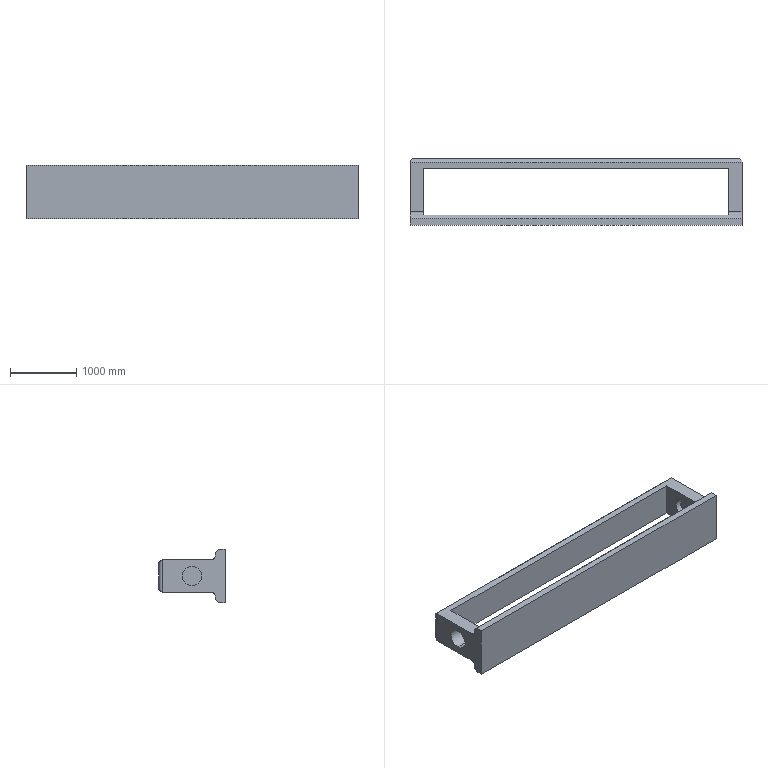Part | SolidWorks | features ICE 4, Attribute 2, Fillet 2, Chamfer 1, Extrusion 1, WeldmentFeature 1 | 1 solid | 27 faces | box 5000 x 1000 x 800 mm | volume 1070403912 mm3 | plane 17 | cylinder 10 | commonest cylinder face diameters 100 x6 290 x2 300 x2
STEP:
#1=CARTESIAN_POINT('',(4890.,500.,150.));
#2=VERTEX_POINT('',#1);
#3=CARTESIAN_POINT('',(4890.,500.,-150.));
#4=VERTEX_POINT('',#3);
#5=CARTESIAN_POINT('',(4890.,500.,0.));
#6=DIRECTION('',(1.,0.,0.));
#7=DIRECTION('',(0.,0.,-1.));
#8=AXIS2_PLACEMENT_3D('',#5,#6,#7);
#9=CIRCLE('',#8,150.);
#10=EDGE_CURVE('',#2,#4,#9,.T.);
#11=ORIENTED_EDGE('',*,*,#10,.T.);
#12=CARTESIAN_POINT('',(4800.,500.,-150.));
#13=VERTEX_POINT('',#12);
#14=CARTESIAN_POINT('',(4890.,500.,-150.));
#15=DIRECTION('',(-1.,0.,0.));
#16=VECTOR('',#15,1000.);
#17=LINE('',#14,#16);
#18=EDGE_CURVE('',#4,#13,#17,.T.);
#19=ORIENTED_EDGE('',*,*,#18,.T.);
#20=CARTESIAN_POINT('',(4800.,500.,150.));
#21=VERTEX_POINT('',#20);
#22=CARTESIAN_POINT('',(4800.,500.,0.));
#23=DIRECTION('',(1.,0.,0.));
#24=DIRECTION('',(0.,0.,-1.));
#25=AXIS2_PLACEMENT_3D('',#22,#23,#24);
#26=CIRCLE('',#25,150.);
#27=EDGE_CURVE('',#21,#13,#26,.T.);
#28=ORIENTED_EDGE('',*,*,#27,.F.);
#29=CARTESIAN_POINT('',(4890.,500.,150.));
#30=DIRECTION('',(-1.,0.,0.));
#31=VECTOR('',#30,1000.);
#32=LINE('',#29,#31);
#33=EDGE_CURVE('',#2,#21,#32,.T.);
#34=ORIENTED_EDGE('',*,*,#33,.F.);
#35=EDGE_LOOP('',(#11,#19,#28,#34));
#36=FACE_OUTER_BOUND('',#35,.T.);
#37=CARTESIAN_POINT('',(4890.,500.,0.));
#38=DIRECTION('',(-1.,0.,0.));
#39=DIRECTION('',(0.,0.,1.));
#40=AXIS2_PLACEMENT_3D('',#37,#38,#39);
#41=CYLINDRICAL_SURFACE('',#40,150.);
#42=ADVANCED_FACE('',(#36),#41,.F.);
#43=CARTESIAN_POINT('',(200.,500.,145.));
#44=VERTEX_POINT('',#43);
#45=CARTESIAN_POINT('',(200.,500.,-145.));
#46=VERTEX_POINT('',#45);
#47=CARTESIAN_POINT('',(200.,500.,0.));
#48=DIRECTION('',(1.,0.,0.));
#49=DIRECTION('',(0.,0.,1.));
#50=AXIS2_PLACEMENT_3D('',#47,#48,#49);
#51=CIRCLE('',#50,145.);
#52=EDGE_CURVE('',#44,#46,#51,.T.);
#53=ORIENTED_EDGE('',*,*,#52,.T.);
#54=CARTESIAN_POINT('',(0.,500.,-145.));
#55=VERTEX_POINT('',#54);
#56=CARTESIAN_POINT('',(610.122,500.,-145.));
#57=DIRECTION('',(-1.,0.,0.));
#58=VECTOR('',#57,1000.);
#59=LINE('',#56,#58);
#60=EDGE_CURVE('',#46,#55,#59,.T.);
#61=ORIENTED_EDGE('',*,*,#60,.T.);
#62=CARTESIAN_POINT('',(0.,500.,145.));
#63=VERTEX_POINT('',#62);
#64=CARTESIAN_POINT('',(0.,500.,0.));
#65=DIRECTION('',(1.,0.,0.));
#66=DIRECTION('',(0.,0.,-1.));
#67=AXIS2_PLACEMENT_3D('',#64,#65,#66);
#68=CIRCLE('',#67,145.);
#69=EDGE_CURVE('',#63,#55,#68,.T.);
#70=ORIENTED_EDGE('',*,*,#69,.F.);
#71=CARTESIAN_POINT('',(610.122,500.,145.));
#72=DIRECTION('',(-1.,0.,0.));
#73=VECTOR('',#72,1000.);
#74=LINE('',#71,#73);
#75=EDGE_CURVE('',#44,#63,#74,.T.);
#76=ORIENTED_EDGE('',*,*,#75,.F.);
#77=EDGE_LOOP('',(#53,#61,#70,#76));
#78=FACE_OUTER_BOUND('',#77,.T.);
#79=CARTESIAN_POINT('',(610.122,500.,0.));
#80=DIRECTION('',(-1.,0.,0.));
#81=DIRECTION('',(0.,0.,1.));
#82=AXIS2_PLACEMENT_3D('',#79,#80,#81);
#83=CYLINDRICAL_SURFACE('',#82,145.);
#84=ADVANCED_FACE('',(#78),#83,.F.);
#85=CARTESIAN_POINT('',(0.,950.,250.));
#86=VERTEX_POINT('',#85);
#87=CARTESIAN_POINT('',(0.,200.,250.));
#88=VERTEX_POINT('',#87);
#89=CARTESIAN_POINT('',(0.,1000.,250.));
#90=DIRECTION('',(0.,-1.,0.));
#91=VECTOR('',#90,1000.);
#92=LINE('',#89,#91);
#93=EDGE_CURVE('',#86,#88,#92,.T.);
#94=ORIENTED_EDGE('',*,*,#93,.T.);
#95=CARTESIAN_POINT('',(200.,200.,250.));
#96=VERTEX_POINT('',#95);
#97=CARTESIAN_POINT('',(200.,200.,250.));
#98=DIRECTION('',(1.,0.,0.));
#99=VECTOR('',#98,1000.);
#100=LINE('',#97,#99);
#101=EDGE_CURVE('',#88,#96,#100,.T.);
#102=ORIENTED_EDGE('',*,*,#101,.T.);
#103=CARTESIAN_POINT('',(200.,850.,250.));
#104=VERTEX_POINT('',#103);
#105=CARTESIAN_POINT('',(200.,850.,250.));
#106=DIRECTION('',(0.,-1.,0.));
#107=VECTOR('',#106,1000.);
#108=LINE('',#105,#107);
#109=EDGE_CURVE('',#104,#96,#108,.T.);
#110=ORIENTED_EDGE('',*,*,#109,.F.);
#111=CARTESIAN_POINT('',(4800.,850.,250.));
#112=VERTEX_POINT('',#111);
#113=CARTESIAN_POINT('',(4800.,850.,250.));
#114=DIRECTION('',(-1.,0.,0.));
#115=VECTOR('',#114,1000.);
#116=LINE('',#113,#115);
#117=EDGE_CURVE('',#112,#104,#116,.T.);
#118=ORIENTED_EDGE('',*,*,#117,.F.);
#119=CARTESIAN_POINT('',(4800.,200.,250.));
#120=VERTEX_POINT('',#119);
#121=CARTESIAN_POINT('',(4800.,850.,250.));
#122=DIRECTION('',(0.,1.,0.));
#123=VECTOR('',#122,1000.);
#124=LINE('',#121,#123);
#125=EDGE_CURVE('',#120,#112,#124,.T.);
#126=ORIENTED_EDGE('',*,*,#125,.F.);
#127=CARTESIAN_POINT('',(5000.,200.,250.));
#128=VERTEX_POINT('',#127);
#129=CARTESIAN_POINT('',(5000.,200.,250.));
#130=DIRECTION('',(1.,0.,0.));
#131=VECTOR('',#130,1000.);
#132=LINE('',#129,#131);
#133=EDGE_CURVE('',#120,#128,#132,.T.);
#134=ORIENTED_EDGE('',*,*,#133,.T.);
#135=CARTESIAN_POINT('',(5000.,950.,250.));
#136=VERTEX_POINT('',#135);
#137=CARTESIAN_POINT('',(5000.,1000.,250.));
#138=DIRECTION('',(0.,1.,0.));
#139=VECTOR('',#138,1000.);
#140=LINE('',#137,#139);
#141=EDGE_CURVE('',#128,#136,#140,.T.);
#142=ORIENTED_EDGE('',*,*,#141,.T.);
#143=CARTESIAN_POINT('',(0.,950.,250.));
#144=DIRECTION('',(-1.,0.,0.));
#145=VECTOR('',#144,1000.);
#146=LINE('',#143,#145);
#147=EDGE_CURVE('',#136,#86,#146,.T.);
#148=ORIENTED_EDGE('',*,*,#147,.T.);
#149=EDGE_LOOP('',(#94,#102,#110,#118,#126,#134,#142,#148));
#150=FACE_OUTER_BOUND('',#149,.T.);
#151=CARTESIAN_POINT('',(0.,0.,250.));
#152=DIRECTION('',(0.,0.,-1.));
#153=DIRECTION('',(-1.,0.,0.));
#154=AXIS2_PLACEMENT_3D('',#151,#152,#153);
#155=PLANE('',#154);
#156=ADVANCED_FACE('',(#150),#155,.F.);
#157=CARTESIAN_POINT('',(200.,850.,-250.));
#158=VERTEX_POINT('',#157);
#159=CARTESIAN_POINT('',(200.,200.,-250.));
#160=VERTEX_POINT('',#159);
#161=CARTESIAN_POINT('',(200.,850.,-250.));
#162=DIRECTION('',(0.,-1.,0.));
#163=VECTOR('',#162,1000.);
#164=LINE('',#161,#163);
#165=EDGE_CURVE('',#158,#160,#164,.T.);
#166=ORIENTED_EDGE('',*,*,#165,.T.);
#167=CARTESIAN_POINT('',(0.,200.,-250.));
#168=VERTEX_POINT('',#167);
#169=CARTESIAN_POINT('',(0.,200.,-250.));
#170=DIRECTION('',(-1.,0.,0.));
#171=VECTOR('',#170,1000.);
#172=LINE('',#169,#171);
#173=EDGE_CURVE('',#160,#168,#172,.T.);
#174=ORIENTED_EDGE('',*,*,#173,.T.);
#175=CARTESIAN_POINT('',(0.,950.,-250.));
#176=VERTEX_POINT('',#175);
#177=CARTESIAN_POINT('',(0.,1000.,-250.));
#178=DIRECTION('',(0.,-1.,0.));
#179=VECTOR('',#178,1000.);
#180=LINE('',#177,#179);
#181=EDGE_CURVE('',#176,#168,#180,.T.);
#182=ORIENTED_EDGE('',*,*,#181,.F.);
#183=CARTESIAN_POINT('',(5000.,950.,-250.));
#184=VERTEX_POINT('',#183);
#185=CARTESIAN_POINT('',(5000.,950.,-250.));
#186=DIRECTION('',(1.,0.,0.));
#187=VECTOR('',#186,1000.);
#188=LINE('',#185,#187);
#189=EDGE_CURVE('',#176,#184,#188,.T.);
#190=ORIENTED_EDGE('',*,*,#189,.T.);
#191=CARTESIAN_POINT('',(5000.,200.,-250.));
#192=VERTEX_POINT('',#191);
#193=CARTESIAN_POINT('',(5000.,1000.,-250.));
#194=DIRECTION('',(0.,1.,0.));
#195=VECTOR('',#194,1000.);
#196=LINE('',#193,#195);
#197=EDGE_CURVE('',#192,#184,#196,.T.);
#198=ORIENTED_EDGE('',*,*,#197,.F.);
#199=CARTESIAN_POINT('',(4800.,200.,-250.));
#200=VERTEX_POINT('',#199);
#201=CARTESIAN_POINT('',(0.,200.,-250.));
#202=DIRECTION('',(-1.,0.,0.));
#203=VECTOR('',#202,1000.);
#204=LINE('',#201,#203);
#205=EDGE_CURVE('',#192,#200,#204,.T.);
#206=ORIENTED_EDGE('',*,*,#205,.T.);
#207=CARTESIAN_POINT('',(4800.,850.,-250.));
#208=VERTEX_POINT('',#207);
#209=CARTESIAN_POINT('',(4800.,850.,-250.));
#210=DIRECTION('',(0.,1.,0.));
#211=VECTOR('',#210,1000.);
#212=LINE('',#209,#211);
#213=EDGE_CURVE('',#200,#208,#212,.T.);
#214=ORIENTED_EDGE('',*,*,#213,.T.);
#215=CARTESIAN_POINT('',(4800.,850.,-250.));
#216=DIRECTION('',(-1.,0.,0.));
#217=VECTOR('',#216,1000.);
#218=LINE('',#215,#217);
#219=EDGE_CURVE('',#208,#158,#218,.T.);
#220=ORIENTED_EDGE('',*,*,#219,.T.);
#221=EDGE_LOOP('',(#166,#174,#182,#190,#198,#206,#214,#220));
#222=FACE_OUTER_BOUND('',#221,.T.);
#223=CARTESIAN_POINT('',(0.,0.,-250.));
#224=DIRECTION('',(0.,0.,-1.));
#225=DIRECTION('',(-1.,0.,0.));
#226=AXIS2_PLACEMENT_3D('',#223,#224,#225);
#227=PLANE('',#226);
#228=ADVANCED_FACE('',(#222),#227,.T.);
#229=ORIENTED_EDGE('',*,*,#197,.T.);
#230=CARTESIAN_POINT('',(5000.,950.,250.));
#231=DIRECTION('',(0.,0.,1.));
#232=VECTOR('',#231,1000.);
#233=LINE('',#230,#232);
#234=EDGE_CURVE('',#184,#136,#233,.T.);
#235=ORIENTED_EDGE('',*,*,#234,.T.);
#236=ORIENTED_EDGE('',*,*,#141,.F.);
#237=CARTESIAN_POINT('',(5000.,150.,300.));
#238=VERTEX_POINT('',#237);
#239=CARTESIAN_POINT('',(5000.,200.,300.));
#240=DIRECTION('',(-1.,0.,0.));
#241=DIRECTION('',(0.,0.,1.));
#242=AXIS2_PLACEMENT_3D('',#239,#240,#241);
#243=CIRCLE('',#242,50.);
#244=EDGE_CURVE('',#128,#238,#243,.T.);
#245=ORIENTED_EDGE('',*,*,#244,.T.);
#246=CARTESIAN_POINT('',(5000.,150.,350.));
#247=VERTEX_POINT('',#246);
#248=CARTESIAN_POINT('',(5000.,150.,400.));
#249=DIRECTION('',(0.,0.,-1.));
#250=VECTOR('',#249,1000.);
#251=LINE('',#248,#250);
#252=EDGE_CURVE('',#247,#238,#251,.T.);
#253=ORIENTED_EDGE('',*,*,#252,.F.);
#254=CARTESIAN_POINT('',(5000.,100.,400.));
#255=VERTEX_POINT('',#254);
#256=CARTESIAN_POINT('',(5000.,150.,350.));
#257=DIRECTION('',(0.,-0.7071,0.7071));
#258=VECTOR('',#257,1000.);
#259=LINE('',#256,#258);
#260=EDGE_CURVE('',#247,#255,#259,.T.);
#261=ORIENTED_EDGE('',*,*,#260,.T.);
#262=CARTESIAN_POINT('',(5000.,0.,400.));
#263=VERTEX_POINT('',#262);
#264=CARTESIAN_POINT('',(5000.,5213.596,400.));
#265=DIRECTION('',(0.,-1.,0.));
#266=VECTOR('',#265,1000.);
#267=LINE('',#264,#266);
#268=EDGE_CURVE('',#255,#263,#267,.T.);
#269=ORIENTED_EDGE('',*,*,#268,.T.);
#270=CARTESIAN_POINT('',(5000.,0.,-400.));
#271=VERTEX_POINT('',#270);
#272=CARTESIAN_POINT('',(5000.,0.,250.));
#273=DIRECTION('',(0.,0.,-1.));
#274=VECTOR('',#273,1000.);
#275=LINE('',#272,#274);
#276=EDGE_CURVE('',#263,#271,#275,.T.);
#277=ORIENTED_EDGE('',*,*,#276,.T.);
#278=CARTESIAN_POINT('',(5000.,100.,-400.));
#279=VERTEX_POINT('',#278);
#280=CARTESIAN_POINT('',(5000.,5213.596,-400.));
#281=DIRECTION('',(0.,-1.,0.));
#282=VECTOR('',#281,1000.);
#283=LINE('',#280,#282);
#284=EDGE_CURVE('',#279,#271,#283,.T.);
#285=ORIENTED_EDGE('',*,*,#284,.F.);
#286=CARTESIAN_POINT('',(5000.,150.,-350.));
#287=VERTEX_POINT('',#286);
#288=CARTESIAN_POINT('',(5000.,150.,-350.));
#289=DIRECTION('',(0.,0.7071,0.7071));
#290=VECTOR('',#289,1000.);
#291=LINE('',#288,#290);
#292=EDGE_CURVE('',#279,#287,#291,.T.);
#293=ORIENTED_EDGE('',*,*,#292,.T.);
#294=CARTESIAN_POINT('',(5000.,150.,-300.));
#295=VERTEX_POINT('',#294);
#296=CARTESIAN_POINT('',(5000.,150.,400.));
#297=DIRECTION('',(0.,0.,-1.));
#298=VECTOR('',#297,1000.);
#299=LINE('',#296,#298);
#300=EDGE_CURVE('',#295,#287,#299,.T.);
#301=ORIENTED_EDGE('',*,*,#300,.F.);
#302=CARTESIAN_POINT('',(5000.,200.,-300.));
#303=DIRECTION('',(-1.,0.,0.));
#304=DIRECTION('',(0.,0.,1.));
#305=AXIS2_PLACEMENT_3D('',#302,#303,#304);
#306=CIRCLE('',#305,50.);
#307=EDGE_CURVE('',#295,#192,#306,.T.);
#308=ORIENTED_EDGE('',*,*,#307,.T.);
#309=EDGE_LOOP('',(#229,#235,#236,#245,#253,#261,#269,#277,#285,#293,#301,#308));
#310=FACE_OUTER_BOUND('',#309,.T.);
#311=CARTESIAN_POINT('',(5000.,1000.,250.));
#312=DIRECTION('',(-1.,0.,0.));
#313=DIRECTION('',(0.,0.,1.));
#314=AXIS2_PLACEMENT_3D('',#311,#312,#313);
#315=PLANE('',#314);
#316=ADVANCED_FACE('',(#310),#315,.F.);
#317=CARTESIAN_POINT('',(50.,1000.,200.));
#318=VERTEX_POINT('',#317);
#319=CARTESIAN_POINT('',(4950.,1000.,200.));
#320=VERTEX_POINT('',#319);
#321=CARTESIAN_POINT('',(0.,1000.,200.));
#322=DIRECTION('',(1.,0.,0.));
#323=VECTOR('',#322,1000.);
#324=LINE('',#321,#323);
#325=EDGE_CURVE('',#318,#320,#324,.T.);
#326=ORIENTED_EDGE('',*,*,#325,.T.);
#327=CARTESIAN_POINT('',(4950.,1000.,-200.));
#328=VERTEX_POINT('',#327);
#329=CARTESIAN_POINT('',(4950.,1000.,250.));
#330=DIRECTION('',(0.,0.,-1.));
#331=VECTOR('',#330,1000.);
#332=LINE('',#329,#331);
#333=EDGE_CURVE('',#320,#328,#332,.T.);
#334=ORIENTED_EDGE('',*,*,#333,.T.);
#335=CARTESIAN_POINT('',(50.,1000.,-200.));
#336=VERTEX_POINT('',#335);
#337=CARTESIAN_POINT('',(0.,1000.,-200.));
#338=DIRECTION('',(-1.,0.,0.));
#339=VECTOR('',#338,1000.);
#340=LINE('',#337,#339);
#341=EDGE_CURVE('',#328,#336,#340,.T.);
#342=ORIENTED_EDGE('',*,*,#341,.T.);
#343=CARTESIAN_POINT('',(50.,1000.,250.));
#344=DIRECTION('',(0.,0.,1.));
#345=VECTOR('',#344,1000.);
#346=LINE('',#343,#345);
#347=EDGE_CURVE('',#336,#318,#346,.T.);
#348=ORIENTED_EDGE('',*,*,#347,.T.);
#349=EDGE_LOOP('',(#326,#334,#342,#348));
#350=FACE_OUTER_BOUND('',#349,.T.);
#351=CARTESIAN_POINT('',(0.,1000.,250.));
#352=DIRECTION('',(0.,-1.,0.));
#353=DIRECTION('',(0.,0.,-1.));
#354=AXIS2_PLACEMENT_3D('',#351,#352,#353);
#355=PLANE('',#354);
#356=ADVANCED_FACE('',(#350),#355,.F.);
#357=ORIENTED_EDGE('',*,*,#93,.F.);
#358=CARTESIAN_POINT('',(0.,950.,250.));
#359=DIRECTION('',(0.,0.,-1.));
#360=VECTOR('',#359,1000.);
#361=LINE('',#358,#360);
#362=EDGE_CURVE('',#86,#176,#361,.T.);
#363=ORIENTED_EDGE('',*,*,#362,.T.);
#364=ORIENTED_EDGE('',*,*,#181,.T.);
#365=CARTESIAN_POINT('',(0.,150.,-300.));
#366=VERTEX_POINT('',#365);
#367=CARTESIAN_POINT('',(0.,200.,-300.));
#368=DIRECTION('',(1.,0.,0.));
#369=DIRECTION('',(0.,0.,-1.));
#370=AXIS2_PLACEMENT_3D('',#367,#368,#369);
#371=CIRCLE('',#370,50.);
#372=EDGE_CURVE('',#168,#366,#371,.T.);
#373=ORIENTED_EDGE('',*,*,#372,.T.);
#374=CARTESIAN_POINT('',(0.,150.,-350.));
#375=VERTEX_POINT('',#374);
#376=CARTESIAN_POINT('',(0.,150.,400.));
#377=DIRECTION('',(0.,0.,1.));
#378=VECTOR('',#377,1000.);
#379=LINE('',#376,#378);
#380=EDGE_CURVE('',#375,#366,#379,.T.);
#381=ORIENTED_EDGE('',*,*,#380,.F.);
#382=CARTESIAN_POINT('',(0.,100.,-400.));
#383=VERTEX_POINT('',#382);
#384=CARTESIAN_POINT('',(0.,150.,-350.));
#385=DIRECTION('',(0.,-0.7071,-0.7071));
#386=VECTOR('',#385,1000.);
#387=LINE('',#384,#386);
#388=EDGE_CURVE('',#375,#383,#387,.T.);
#389=ORIENTED_EDGE('',*,*,#388,.T.);
#390=CARTESIAN_POINT('',(0.,0.,-400.));
#391=VERTEX_POINT('',#390);
#392=CARTESIAN_POINT('',(0.,5213.596,-400.));
#393=DIRECTION('',(0.,-1.,0.));
#394=VECTOR('',#393,1000.);
#395=LINE('',#392,#394);
#396=EDGE_CURVE('',#383,#391,#395,.T.);
#397=ORIENTED_EDGE('',*,*,#396,.T.);
#398=CARTESIAN_POINT('',(0.,0.,400.));
#399=VERTEX_POINT('',#398);
#400=CARTESIAN_POINT('',(0.,0.,250.));
#401=DIRECTION('',(0.,0.,-1.));
#402=VECTOR('',#401,1000.);
#403=LINE('',#400,#402);
#404=EDGE_CURVE('',#399,#391,#403,.T.);
#405=ORIENTED_EDGE('',*,*,#404,.F.);
#406=CARTESIAN_POINT('',(0.,100.,400.));
#407=VERTEX_POINT('',#406);
#408=CARTESIAN_POINT('',(0.,5213.596,400.));
#409=DIRECTION('',(0.,-1.,0.));
#410=VECTOR('',#409,1000.);
#411=LINE('',#408,#410);
#412=EDGE_CURVE('',#407,#399,#411,.T.);
#413=ORIENTED_EDGE('',*,*,#412,.F.);
#414=CARTESIAN_POINT('',(0.,150.,350.));
#415=VERTEX_POINT('',#414);
#416=CARTESIAN_POINT('',(0.,150.,350.));
#417=DIRECTION('',(0.,0.7071,-0.7071));
#418=VECTOR('',#417,1000.);
#419=LINE('',#416,#418);
#420=EDGE_CURVE('',#407,#415,#419,.T.);
#421=ORIENTED_EDGE('',*,*,#420,.T.);
#422=CARTESIAN_POINT('',(0.,150.,300.));
#423=VERTEX_POINT('',#422);
#424=CARTESIAN_POINT('',(0.,150.,400.));
#425=DIRECTION('',(0.,0.,1.));
#426=VECTOR('',#425,1000.);
#427=LINE('',#424,#426);
#428=EDGE_CURVE('',#423,#415,#427,.T.);
#429=ORIENTED_EDGE('',*,*,#428,.F.);
#430=CARTESIAN_POINT('',(0.,200.,300.));
#431=DIRECTION('',(1.,0.,0.));
#432=DIRECTION('',(0.,0.,-1.));
#433=AXIS2_PLACEMENT_3D('',#430,#431,#432);
#434=CIRCLE('',#433,50.);
#435=EDGE_CURVE('',#423,#88,#434,.T.);
#436=ORIENTED_EDGE('',*,*,#435,.T.);
#437=EDGE_LOOP('',(#357,#363,#364,#373,#381,#389,#397,#405,#413,#421,#429,#436));
#438=FACE_OUTER_BOUND('',#437,.T.);
#439=ORIENTED_EDGE('',*,*,#69,.T.);
#440=CARTESIAN_POINT('',(0.,500.,0.));
#441=DIRECTION('',(1.,0.,0.));
#442=DIRECTION('',(0.,0.,-1.));
#443=AXIS2_PLACEMENT_3D('',#440,#441,#442);
#444=CIRCLE('',#443,145.);
#445=EDGE_CURVE('',#55,#63,#444,.T.);
#446=ORIENTED_EDGE('',*,*,#445,.T.);
#447=EDGE_LOOP('',(#439,#446));
#448=FACE_BOUND('',#447,.T.);
#449=CARTESIAN_POINT('',(0.,1000.,250.));
#450=DIRECTION('',(1.,0.,0.));
#451=DIRECTION('',(0.,0.,-1.));
#452=AXIS2_PLACEMENT_3D('',#449,#450,#451);
#453=PLANE('',#452);
#454=ADVANCED_FACE('',(#438,#448),#453,.F.);
#455=ORIENTED_EDGE('',*,*,#404,.T.);
#456=CARTESIAN_POINT('',(0.,0.,-400.));
#457=DIRECTION('',(1.,0.,0.));
#458=VECTOR('',#457,1000.);
#459=LINE('',#456,#458);
#460=EDGE_CURVE('',#391,#271,#459,.T.);
#461=ORIENTED_EDGE('',*,*,#460,.T.);
#462=ORIENTED_EDGE('',*,*,#276,.F.);
#463=CARTESIAN_POINT('',(0.,0.,400.));
#464=DIRECTION('',(-1.,0.,0.));
#465=VECTOR('',#464,1000.);
#466=LINE('',#463,#465);
#467=EDGE_CURVE('',#263,#399,#466,.T.);
#468=ORIENTED_EDGE('',*,*,#467,.T.);
#469=EDGE_LOOP('',(#455,#461,#462,#468));
#470=FACE_OUTER_BOUND('',#469,.T.);
#471=CARTESIAN_POINT('',(5000.,0.,250.));
#472=DIRECTION('',(0.,1.,0.));
#473=DIRECTION('',(0.,0.,1.));
#474=AXIS2_PLACEMENT_3D('',#471,#472,#473);
#475=PLANE('',#474);
#476=ADVANCED_FACE('',(#470),#475,.F.);
#477=ORIENTED_EDGE('',*,*,#52,.F.);
#478=CARTESIAN_POINT('',(200.,500.,0.));
#479=DIRECTION('',(1.,0.,0.));
#480=DIRECTION('',(0.,0.,1.));
#481=AXIS2_PLACEMENT_3D('',#478,#479,#480);
#482=CIRCLE('',#481,145.);
#483=EDGE_CURVE('',#46,#44,#482,.T.);
#484=ORIENTED_EDGE('',*,*,#483,.F.);
#485=EDGE_LOOP('',(#477,#484));
#486=FACE_BOUND('',#485,.T.);
#487=ORIENTED_EDGE('',*,*,#109,.T.);
#488=CARTESIAN_POINT('',(200.,150.,300.));
#489=VERTEX_POINT('',#488);
#490=CARTESIAN_POINT('',(200.,200.,300.));
#491=DIRECTION('',(-1.,0.,0.));
#492=DIRECTION('',(0.,0.,1.));
#493=AXIS2_PLACEMENT_3D('',#490,#491,#492);
#494=CIRCLE('',#493,50.);
#495=EDGE_CURVE('',#96,#489,#494,.T.);
#496=ORIENTED_EDGE('',*,*,#495,.T.);
#497=CARTESIAN_POINT('',(200.,150.,-300.));
#498=VERTEX_POINT('',#497);
#499=CARTESIAN_POINT('',(200.,150.,-250.));
#500=DIRECTION('',(0.,0.,1.));
#501=VECTOR('',#500,1000.);
#502=LINE('',#499,#501);
#503=EDGE_CURVE('',#498,#489,#502,.T.);
#504=ORIENTED_EDGE('',*,*,#503,.F.);
#505=CARTESIAN_POINT('',(200.,200.,-300.));
#506=DIRECTION('',(-1.,0.,0.));
#507=DIRECTION('',(0.,0.,1.));
#508=AXIS2_PLACEMENT_3D('',#505,#506,#507);
#509=CIRCLE('',#508,50.);
#510=EDGE_CURVE('',#498,#160,#509,.T.);
#511=ORIENTED_EDGE('',*,*,#510,.T.);
#512=ORIENTED_EDGE('',*,*,#165,.F.);
#513=CARTESIAN_POINT('',(200.,850.,-250.));
#514=DIRECTION('',(0.,0.,1.));
#515=VECTOR('',#514,1000.);
#516=LINE('',#513,#515);
#517=EDGE_CURVE('',#158,#104,#516,.T.);
#518=ORIENTED_EDGE('',*,*,#517,.T.);
#519=EDGE_LOOP('',(#487,#496,#504,#511,#512,#518));
#520=FACE_OUTER_BOUND('',#519,.T.);
#521=CARTESIAN_POINT('',(200.,850.,-250.));
#522=DIRECTION('',(-1.,0.,0.));
#523=DIRECTION('',(0.,0.,1.));
#524=AXIS2_PLACEMENT_3D('',#521,#522,#523);
#525=PLANE('',#524);
#526=ADVANCED_FACE('',(#486,#520),#525,.F.);
#527=ORIENTED_EDGE('',*,*,#117,.T.);
#528=ORIENTED_EDGE('',*,*,#517,.F.);
#529=ORIENTED_EDGE('',*,*,#219,.F.);
#530=CARTESIAN_POINT('',(4800.,850.,-250.));
#531=DIRECTION('',(0.,0.,1.));
#532=VECTOR('',#531,1000.);
#533=LINE('',#530,#532);
#534=EDGE_CURVE('',#208,#112,#533,.T.);
#535=ORIENTED_EDGE('',*,*,#534,.T.);
#536=EDGE_LOOP('',(#527,#528,#529,#535));
#537=FACE_OUTER_BOUND('',#536,.T.);
#538=CARTESIAN_POINT('',(4800.,850.,-250.));
#539=DIRECTION('',(0.,1.,0.));
#540=DIRECTION('',(0.,0.,1.));
#541=AXIS2_PLACEMENT_3D('',#538,#539,#540);
#542=PLANE('',#541);
#543=ADVANCED_FACE('',(#537),#542,.F.);
#544=ORIENTED_EDGE('',*,*,#27,.T.);
#545=CARTESIAN_POINT('',(4800.,500.,0.));
#546=DIRECTION('',(1.,0.,0.));
#547=DIRECTION('',(0.,0.,-1.));
#548=AXIS2_PLACEMENT_3D('',#545,#546,#547);
#549=CIRCLE('',#548,150.);
#550=EDGE_CURVE('',#13,#21,#549,.T.);
#551=ORIENTED_EDGE('',*,*,#550,.T.);
#552=EDGE_LOOP('',(#544,#551));
#553=FACE_BOUND('',#552,.T.);
#554=CARTESIAN_POINT('',(4800.,150.,-300.));
#555=VERTEX_POINT('',#554);
#556=CARTESIAN_POINT('',(4800.,150.,300.));
#557=VERTEX_POINT('',#556);
#558=CARTESIAN_POINT('',(4800.,150.,-250.));
#559=DIRECTION('',(0.,0.,1.));
#560=VECTOR('',#559,1000.);
#561=LINE('',#558,#560);
#562=EDGE_CURVE('',#555,#557,#561,.T.);
#563=ORIENTED_EDGE('',*,*,#562,.T.);
#564=CARTESIAN_POINT('',(4800.,200.,300.));
#565=DIRECTION('',(1.,0.,0.));
#566=DIRECTION('',(0.,0.,-1.));
#567=AXIS2_PLACEMENT_3D('',#564,#565,#566);
#568=CIRCLE('',#567,50.);
#569=EDGE_CURVE('',#557,#120,#568,.T.);
#570=ORIENTED_EDGE('',*,*,#569,.T.);
#571=ORIENTED_EDGE('',*,*,#125,.T.);
#572=ORIENTED_EDGE('',*,*,#534,.F.);
#573=ORIENTED_EDGE('',*,*,#213,.F.);
#574=CARTESIAN_POINT('',(4800.,200.,-300.));
#575=DIRECTION('',(1.,0.,0.));
#576=DIRECTION('',(0.,0.,-1.));
#577=AXIS2_PLACEMENT_3D('',#574,#575,#576);
#578=CIRCLE('',#577,50.);
#579=EDGE_CURVE('',#200,#555,#578,.T.);
#580=ORIENTED_EDGE('',*,*,#579,.T.);
#581=EDGE_LOOP('',(#563,#570,#571,#572,#573,#580));
#582=FACE_OUTER_BOUND('',#581,.T.);
#583=CARTESIAN_POINT('',(4800.,850.,-250.));
#584=DIRECTION('',(1.,0.,0.));
#585=DIRECTION('',(0.,0.,-1.));
#586=AXIS2_PLACEMENT_3D('',#583,#584,#585);
#587=PLANE('',#586);
#588=ADVANCED_FACE('',(#553,#582),#587,.F.);
#589=ORIENTED_EDGE('',*,*,#380,.T.);
#590=CARTESIAN_POINT('',(4800.,150.,-300.));
#591=DIRECTION('',(1.,0.,0.));
#592=VECTOR('',#591,1000.);
#593=LINE('',#590,#592);
#594=EDGE_CURVE('',#366,#498,#593,.T.);
#595=ORIENTED_EDGE('',*,*,#594,.T.);
#596=ORIENTED_EDGE('',*,*,#503,.T.);
#597=CARTESIAN_POINT('',(0.,150.,300.));
#598=DIRECTION('',(-1.,0.,0.));
#599=VECTOR('',#598,1000.);
#600=LINE('',#597,#599);
#601=EDGE_CURVE('',#489,#423,#600,.T.);
#602=ORIENTED_EDGE('',*,*,#601,.T.);
#603=ORIENTED_EDGE('',*,*,#428,.T.);
#604=CARTESIAN_POINT('',(5000.,150.,350.));
#605=DIRECTION('',(1.,0.,0.));
#606=VECTOR('',#605,1000.);
#607=LINE('',#604,#606);
#608=EDGE_CURVE('',#415,#247,#607,.T.);
#609=ORIENTED_EDGE('',*,*,#608,.T.);
#610=ORIENTED_EDGE('',*,*,#252,.T.);
#611=CARTESIAN_POINT('',(4800.,150.,300.));
#612=DIRECTION('',(-1.,0.,0.));
#613=VECTOR('',#612,1000.);
#614=LINE('',#611,#613);
#615=EDGE_CURVE('',#238,#557,#614,.T.);
#616=ORIENTED_EDGE('',*,*,#615,.T.);
#617=ORIENTED_EDGE('',*,*,#562,.F.);
#618=CARTESIAN_POINT('',(4800.,150.,-300.));
#619=DIRECTION('',(1.,0.,0.));
#620=VECTOR('',#619,1000.);
#621=LINE('',#618,#620);
#622=EDGE_CURVE('',#555,#295,#621,.T.);
#623=ORIENTED_EDGE('',*,*,#622,.T.);
#624=ORIENTED_EDGE('',*,*,#300,.T.);
#625=CARTESIAN_POINT('',(0.,150.,-350.));
#626=DIRECTION('',(-1.,0.,0.));
#627=VECTOR('',#626,1000.);
#628=LINE('',#625,#627);
#629=EDGE_CURVE('',#287,#375,#628,.T.);
#630=ORIENTED_EDGE('',*,*,#629,.T.);
#631=EDGE_LOOP('',(#589,#595,#596,#602,#603,#609,#610,#616,#617,#623,#624,#630));
#632=FACE_OUTER_BOUND('',#631,.T.);
#633=CARTESIAN_POINT('',(4800.,150.,-250.));
#634=DIRECTION('',(0.,-1.,0.));
#635=DIRECTION('',(0.,0.,-1.));
#636=AXIS2_PLACEMENT_3D('',#633,#634,#635);
#637=PLANE('',#636);
#638=ADVANCED_FACE('',(#632),#637,.F.);
#639=ORIENTED_EDGE('',*,*,#60,.F.);
#640=ORIENTED_EDGE('',*,*,#483,.T.);
#641=ORIENTED_EDGE('',*,*,#75,.T.);
#642=ORIENTED_EDGE('',*,*,#445,.F.);
#643=EDGE_LOOP('',(#639,#640,#641,#642));
#644=FACE_OUTER_BOUND('',#643,.T.);
#645=CARTESIAN_POINT('',(610.122,500.,0.));
#646=DIRECTION('',(-1.,0.,0.));
#647=DIRECTION('',(0.,0.,1.));
#648=AXIS2_PLACEMENT_3D('',#645,#646,#647);
#649=CYLINDRICAL_SURFACE('',#648,145.);
#650=ADVANCED_FACE('',(#644),#649,.F.);
#651=ORIENTED_EDGE('',*,*,#396,.F.);
#652=CARTESIAN_POINT('',(5000.,100.,-400.));
#653=DIRECTION('',(1.,0.,0.));
#654=VECTOR('',#653,1000.);
#655=LINE('',#652,#654);
#656=EDGE_CURVE('',#383,#279,#655,.T.);
#657=ORIENTED_EDGE('',*,*,#656,.T.);
#658=ORIENTED_EDGE('',*,*,#284,.T.);
#659=ORIENTED_EDGE('',*,*,#460,.F.);
#660=EDGE_LOOP('',(#651,#657,#658,#659));
#661=FACE_OUTER_BOUND('',#660,.T.);
#662=CARTESIAN_POINT('',(0.,5213.596,-400.));
#663=DIRECTION('',(0.,0.,-1.));
#664=DIRECTION('',(-1.,0.,0.));
#665=AXIS2_PLACEMENT_3D('',#662,#663,#664);
#666=PLANE('',#665);
#667=ADVANCED_FACE('',(#661),#666,.T.);
#668=ORIENTED_EDGE('',*,*,#268,.F.);
#669=CARTESIAN_POINT('',(0.,100.,400.));
#670=DIRECTION('',(-1.,0.,0.));
#671=VECTOR('',#670,1000.);
#672=LINE('',#669,#671);
#673=EDGE_CURVE('',#255,#407,#672,.T.);
#674=ORIENTED_EDGE('',*,*,#673,.T.);
#675=ORIENTED_EDGE('',*,*,#412,.T.);
#676=ORIENTED_EDGE('',*,*,#467,.F.);
#677=EDGE_LOOP('',(#668,#674,#675,#676));
#678=FACE_OUTER_BOUND('',#677,.T.);
#679=CARTESIAN_POINT('',(0.,5213.596,400.));
#680=DIRECTION('',(0.,0.,1.));
#681=DIRECTION('',(1.,0.,0.));
#682=AXIS2_PLACEMENT_3D('',#679,#680,#681);
#683=PLANE('',#682);
#684=ADVANCED_FACE('',(#678),#683,.T.);
#685=ORIENTED_EDGE('',*,*,#341,.F.);
#686=CARTESIAN_POINT('',(4950.,1000.,-200.));
#687=CARTESIAN_POINT('',(4979.289,1000.,-200.));
#688=CARTESIAN_POINT('',(5000.,979.289,-220.711));
#689=CARTESIAN_POINT('',(5000.,950.,-250.));
#690=(BOUNDED_CURVE()B_SPLINE_CURVE(3,(#686,#687,#688,#689),.UNSPECIFIED.,.F.,.T.)B_SPLINE_CURVE_WITH_KNOTS((4,4),(3.142,4.712),.UNSPECIFIED.)CURVE()GEOMETRIC_REPRESENTATION_ITEM()RATIONAL_B_SPLINE_CURVE((1.,0.8047,0.8047,1.))REPRESENTATION_ITEM(''));
#691=EDGE_CURVE('',#328,#184,#690,.T.);
#692=ORIENTED_EDGE('',*,*,#691,.T.);
#693=ORIENTED_EDGE('',*,*,#189,.F.);
#694=CARTESIAN_POINT('',(0.,950.,-250.));
#695=CARTESIAN_POINT('',(0.,979.289,-220.711));
#696=CARTESIAN_POINT('',(20.711,1000.,-200.));
#697=CARTESIAN_POINT('',(50.,1000.,-200.));
#698=(BOUNDED_CURVE()B_SPLINE_CURVE(3,(#694,#695,#696,#697),.UNSPECIFIED.,.F.,.F.)B_SPLINE_CURVE_WITH_KNOTS((4,4),(1.571,3.142),.UNSPECIFIED.)CURVE()GEOMETRIC_REPRESENTATION_ITEM()RATIONAL_B_SPLINE_CURVE((1.,0.8047,0.8047,1.))REPRESENTATION_ITEM(''));
#699=EDGE_CURVE('',#176,#336,#698,.T.);
#700=ORIENTED_EDGE('',*,*,#699,.T.);
#701=EDGE_LOOP('',(#685,#692,#693,#700));
#702=FACE_OUTER_BOUND('',#701,.T.);
#703=CARTESIAN_POINT('',(0.,1000.,-200.));
#704=DIRECTION('',(0.,0.7071,-0.7071));
#705=DIRECTION('',(1.,0.,0.));
#706=AXIS2_PLACEMENT_3D('',#703,#704,#705);
#707=PLANE('',#706);
#708=ADVANCED_FACE('',(#702),#707,.T.);
#709=ORIENTED_EDGE('',*,*,#147,.F.);
#710=CARTESIAN_POINT('',(5000.,950.,250.));
#711=CARTESIAN_POINT('',(5000.,979.289,220.711));
#712=CARTESIAN_POINT('',(4979.289,1000.,200.));
#713=CARTESIAN_POINT('',(4950.,1000.,200.));
#714=(BOUNDED_CURVE()B_SPLINE_CURVE(3,(#710,#711,#712,#713),.UNSPECIFIED.,.F.,.F.)B_SPLINE_CURVE_WITH_KNOTS((4,4),(4.712,6.283),.UNSPECIFIED.)CURVE()GEOMETRIC_REPRESENTATION_ITEM()RATIONAL_B_SPLINE_CURVE((1.,0.8047,0.8047,1.))REPRESENTATION_ITEM(''));
#715=EDGE_CURVE('',#136,#320,#714,.T.);
#716=ORIENTED_EDGE('',*,*,#715,.T.);
#717=ORIENTED_EDGE('',*,*,#325,.F.);
#718=CARTESIAN_POINT('',(50.,1000.,200.));
#719=CARTESIAN_POINT('',(20.711,1000.,200.));
#720=CARTESIAN_POINT('',(0.,979.289,220.711));
#721=CARTESIAN_POINT('',(0.,950.,250.));
#722=(BOUNDED_CURVE()B_SPLINE_CURVE(3,(#718,#719,#720,#721),.UNSPECIFIED.,.F.,.T.)B_SPLINE_CURVE_WITH_KNOTS((4,4),(0.,1.571),.UNSPECIFIED.)CURVE()GEOMETRIC_REPRESENTATION_ITEM()RATIONAL_B_SPLINE_CURVE((1.,0.8047,0.8047,1.))REPRESENTATION_ITEM(''));
#723=EDGE_CURVE('',#318,#86,#722,.T.);
#724=ORIENTED_EDGE('',*,*,#723,.T.);
#725=EDGE_LOOP('',(#709,#716,#717,#724));
#726=FACE_OUTER_BOUND('',#725,.T.);
#727=CARTESIAN_POINT('',(0.,950.,250.));
#728=DIRECTION('',(0.,-0.7071,-0.7071));
#729=DIRECTION('',(-1.,0.,0.));
#730=AXIS2_PLACEMENT_3D('',#727,#728,#729);
#731=PLANE('',#730);
#732=ADVANCED_FACE('',(#726),#731,.F.);
#733=ORIENTED_EDGE('',*,*,#420,.F.);
#734=ORIENTED_EDGE('',*,*,#673,.F.);
#735=ORIENTED_EDGE('',*,*,#260,.F.);
#736=ORIENTED_EDGE('',*,*,#608,.F.);
#737=EDGE_LOOP('',(#733,#734,#735,#736));
#738=FACE_OUTER_BOUND('',#737,.T.);
#739=CARTESIAN_POINT('',(4800.,150.,350.));
#740=DIRECTION('',(0.,0.7071,0.7071));
#741=DIRECTION('',(-1.,0.,0.));
#742=AXIS2_PLACEMENT_3D('',#739,#740,#741);
#743=PLANE('',#742);
#744=ADVANCED_FACE('',(#738),#743,.T.);
#745=ORIENTED_EDGE('',*,*,#292,.F.);
#746=ORIENTED_EDGE('',*,*,#656,.F.);
#747=ORIENTED_EDGE('',*,*,#388,.F.);
#748=ORIENTED_EDGE('',*,*,#629,.F.);
#749=EDGE_LOOP('',(#745,#746,#747,#748));
#750=FACE_OUTER_BOUND('',#749,.T.);
#751=CARTESIAN_POINT('',(4800.,150.,-350.));
#752=DIRECTION('',(0.,0.7071,-0.7071));
#753=DIRECTION('',(1.,0.,0.));
#754=AXIS2_PLACEMENT_3D('',#751,#752,#753);
#755=PLANE('',#754);
#756=ADVANCED_FACE('',(#750),#755,.T.);
#757=ORIENTED_EDGE('',*,*,#510,.F.);
#758=ORIENTED_EDGE('',*,*,#594,.F.);
#759=ORIENTED_EDGE('',*,*,#372,.F.);
#760=ORIENTED_EDGE('',*,*,#173,.F.);
#761=EDGE_LOOP('',(#757,#758,#759,#760));
#762=FACE_OUTER_BOUND('',#761,.T.);
#763=CARTESIAN_POINT('',(0.,200.,-300.));
#764=DIRECTION('',(-1.,0.,0.));
#765=DIRECTION('',(0.,0.,1.));
#766=AXIS2_PLACEMENT_3D('',#763,#764,#765);
#767=CYLINDRICAL_SURFACE('',#766,50.);
#768=ADVANCED_FACE('',(#762),#767,.F.);
#769=ORIENTED_EDGE('',*,*,#495,.F.);
#770=ORIENTED_EDGE('',*,*,#101,.F.);
#771=ORIENTED_EDGE('',*,*,#435,.F.);
#772=ORIENTED_EDGE('',*,*,#601,.F.);
#773=EDGE_LOOP('',(#769,#770,#771,#772));
#774=FACE_OUTER_BOUND('',#773,.T.);
#775=CARTESIAN_POINT('',(4800.,200.,300.));
#776=DIRECTION('',(1.,0.,0.));
#777=DIRECTION('',(0.,0.,-1.));
#778=AXIS2_PLACEMENT_3D('',#775,#776,#777);
#779=CYLINDRICAL_SURFACE('',#778,50.);
#780=ADVANCED_FACE('',(#774),#779,.F.);
#781=ORIENTED_EDGE('',*,*,#244,.F.);
#782=ORIENTED_EDGE('',*,*,#133,.F.);
#783=ORIENTED_EDGE('',*,*,#569,.F.);
#784=ORIENTED_EDGE('',*,*,#615,.F.);
#785=EDGE_LOOP('',(#781,#782,#783,#784));
#786=FACE_OUTER_BOUND('',#785,.T.);
#787=CARTESIAN_POINT('',(4800.,200.,300.));
#788=DIRECTION('',(1.,0.,0.));
#789=DIRECTION('',(0.,0.,-1.));
#790=AXIS2_PLACEMENT_3D('',#787,#788,#789);
#791=CYLINDRICAL_SURFACE('',#790,50.);
#792=ADVANCED_FACE('',(#786),#791,.F.);
#793=ORIENTED_EDGE('',*,*,#307,.F.);
#794=ORIENTED_EDGE('',*,*,#622,.F.);
#795=ORIENTED_EDGE('',*,*,#579,.F.);
#796=ORIENTED_EDGE('',*,*,#205,.F.);
#797=EDGE_LOOP('',(#793,#794,#795,#796));
#798=FACE_OUTER_BOUND('',#797,.T.);
#799=CARTESIAN_POINT('',(0.,200.,-300.));
#800=DIRECTION('',(-1.,0.,0.));
#801=DIRECTION('',(0.,0.,1.));
#802=AXIS2_PLACEMENT_3D('',#799,#800,#801);
#803=CYLINDRICAL_SURFACE('',#802,50.);
#804=ADVANCED_FACE('',(#798),#803,.F.);
#805=ORIENTED_EDGE('',*,*,#715,.F.);
#806=ORIENTED_EDGE('',*,*,#234,.F.);
#807=ORIENTED_EDGE('',*,*,#691,.F.);
#808=ORIENTED_EDGE('',*,*,#333,.F.);
#809=EDGE_LOOP('',(#805,#806,#807,#808));
#810=FACE_OUTER_BOUND('',#809,.T.);
#811=CARTESIAN_POINT('',(4950.,950.,250.));
#812=DIRECTION('',(0.,0.,-1.));
#813=DIRECTION('',(-1.,0.,0.));
#814=AXIS2_PLACEMENT_3D('',#811,#812,#813);
#815=CYLINDRICAL_SURFACE('',#814,50.);
#816=ADVANCED_FACE('',(#810),#815,.T.);
#817=ORIENTED_EDGE('',*,*,#723,.F.);
#818=ORIENTED_EDGE('',*,*,#347,.F.);
#819=ORIENTED_EDGE('',*,*,#699,.F.);
#820=ORIENTED_EDGE('',*,*,#362,.F.);
#821=EDGE_LOOP('',(#817,#818,#819,#820));
#822=FACE_OUTER_BOUND('',#821,.T.);
#823=CARTESIAN_POINT('',(50.,950.,250.));
#824=DIRECTION('',(0.,0.,-1.));
#825=DIRECTION('',(-1.,0.,0.));
#826=AXIS2_PLACEMENT_3D('',#823,#824,#825);
#827=CYLINDRICAL_SURFACE('',#826,50.);
#828=ADVANCED_FACE('',(#822),#827,.T.);
#829=ORIENTED_EDGE('',*,*,#18,.F.);
#830=CARTESIAN_POINT('',(4890.,500.,0.));
#831=DIRECTION('',(1.,0.,0.));
#832=DIRECTION('',(0.,0.,-1.));
#833=AXIS2_PLACEMENT_3D('',#830,#831,#832);
#834=CIRCLE('',#833,150.);
#835=EDGE_CURVE('',#4,#2,#834,.T.);
#836=ORIENTED_EDGE('',*,*,#835,.T.);
#837=ORIENTED_EDGE('',*,*,#33,.T.);
#838=ORIENTED_EDGE('',*,*,#550,.F.);
#839=EDGE_LOOP('',(#829,#836,#837,#838));
#840=FACE_OUTER_BOUND('',#839,.T.);
#841=CARTESIAN_POINT('',(4890.,500.,0.));
#842=DIRECTION('',(-1.,0.,0.));
#843=DIRECTION('',(0.,0.,1.));
#844=AXIS2_PLACEMENT_3D('',#841,#842,#843);
#845=CYLINDRICAL_SURFACE('',#844,150.);
#846=ADVANCED_FACE('',(#840),#845,.F.);
#847=ORIENTED_EDGE('',*,*,#10,.F.);
#848=ORIENTED_EDGE('',*,*,#835,.F.);
#849=EDGE_LOOP('',(#847,#848));
#850=FACE_OUTER_BOUND('',#849,.T.);
#851=CARTESIAN_POINT('',(4890.,500.,0.));
#852=DIRECTION('',(1.,0.,0.));
#853=DIRECTION('',(0.,0.,-1.));
#854=AXIS2_PLACEMENT_3D('',#851,#852,#853);
#855=PLANE('',#854);
#856=ADVANCED_FACE('',(#850),#855,.F.);
#857=CLOSED_SHELL('',(#42,#84,#156,#228,#316,#356,#454,#476,#526,#543,#588,#638,#650,#667,#684,#708,#732,#744,#756,#768,#780,#792,#804,#816,#828,#846,#856));
#858=MANIFOLD_SOLID_BREP('',#857);
#859=CARTESIAN_POINT('',(0.,0.,0.));
#860=DIRECTION('',(0.,0.,1.));
#861=DIRECTION('',(1.,0.,0.));
#862=AXIS2_PLACEMENT_3D('',#859,#860,#861);
#863=(LENGTH_UNIT()NAMED_UNIT(*)SI_UNIT(.MILLI.,.METRE.));
#864=UNCERTAINTY_MEASURE_WITH_UNIT(LENGTH_MEASURE(0.00001),#863,'','');
#865=(NAMED_UNIT(*)PLANE_ANGLE_UNIT()SI_UNIT($,.RADIAN.));
#866=(NAMED_UNIT(*)SI_UNIT($,.STERADIAN.)SOLID_ANGLE_UNIT());
#867=(GEOMETRIC_REPRESENTATION_CONTEXT(3)GLOBAL_UNCERTAINTY_ASSIGNED_CONTEXT((#864))GLOBAL_UNIT_ASSIGNED_CONTEXT((#863,#865,#866))REPRESENTATION_CONTEXT('',''));
#868=ADVANCED_BREP_SHAPE_REPRESENTATION('',(#858,#862),#867);